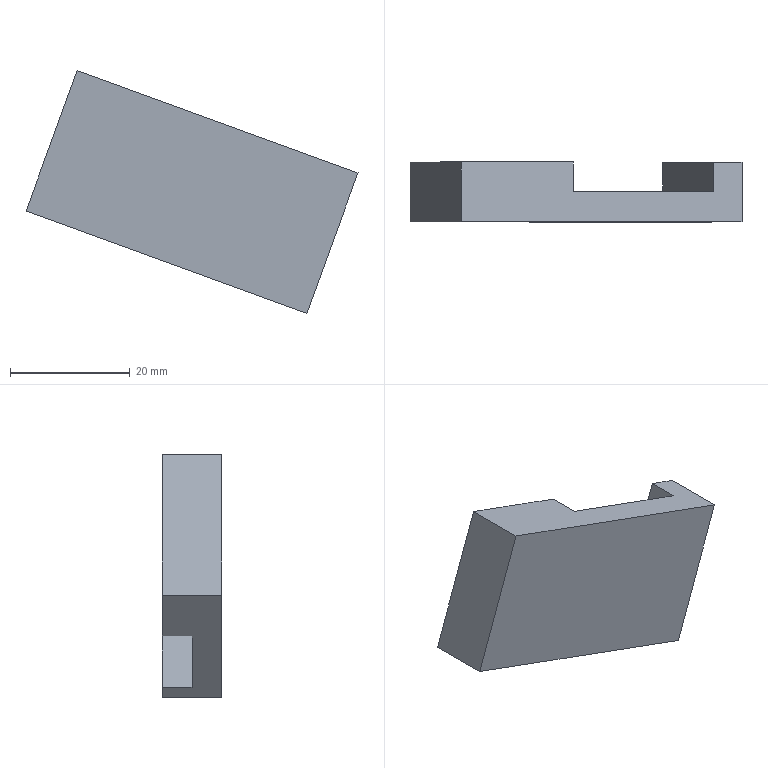Part | NX | features solid 2 | 1 solid | 10 faces | box 55.535 x 10 x 40.593 mm | volume 9375 mm3 | plane 10
STEP:
#1=CARTESIAN_POINT('',(816.611,435.,73.868));
#2=VERTEX_POINT('',#1);
#3=CARTESIAN_POINT('',(825.161,435.,97.361));
#4=VERTEX_POINT('',#3);
#5=CARTESIAN_POINT('',(822.425,435.,89.843));
#6=DIRECTION('',(-0.342,0.,-0.9397));
#7=VECTOR('',#6,1000.);
#8=LINE('',#5,#7);
#9=EDGE_CURVE('',#2,#4,#8,.F.);
#10=ORIENTED_EDGE('',*,*,#9,.T.);
#11=CARTESIAN_POINT('',(829.86,435.,95.651));
#12=VERTEX_POINT('',#11);
#13=CARTESIAN_POINT('',(782.875,435.,112.752));
#14=DIRECTION('',(-0.9397,0.,0.342));
#15=VECTOR('',#14,1000.);
#16=LINE('',#13,#15);
#17=EDGE_CURVE('',#4,#12,#16,.F.);
#18=ORIENTED_EDGE('',*,*,#17,.T.);
#19=CARTESIAN_POINT('',(821.309,435.,72.158));
#20=VERTEX_POINT('',#19);
#21=CARTESIAN_POINT('',(827.124,435.,88.133));
#22=DIRECTION('',(0.342,0.,0.9397));
#23=VECTOR('',#22,1000.);
#24=LINE('',#21,#23);
#25=EDGE_CURVE('',#12,#20,#24,.F.);
#26=ORIENTED_EDGE('',*,*,#25,.T.);
#27=CARTESIAN_POINT('',(774.325,435.,89.259));
#28=DIRECTION('',(-0.9397,0.,0.342));
#29=VECTOR('',#28,1000.);
#30=LINE('',#27,#29);
#31=EDGE_CURVE('',#2,#20,#30,.F.);
#32=ORIENTED_EDGE('',*,*,#31,.F.);
#33=EDGE_LOOP('',(#10,#18,#26,#32));
#34=FACE_BOUND('',#33,.T.);
#35=CARTESIAN_POINT('',(780.139,435.,105.234));
#36=DIRECTION('',(0.,-1.,0.));
#37=DIRECTION('',(0.9397,0.,-0.342));
#38=AXIS2_PLACEMENT_3D('',#35,#36,#37);
#39=PLANE('',#38);
#40=ADVANCED_FACE('',(#34),#39,.F.);
#41=CARTESIAN_POINT('',(782.875,425.,112.752));
#42=VERTEX_POINT('',#41);
#43=CARTESIAN_POINT('',(774.325,425.,89.259));
#44=VERTEX_POINT('',#43);
#45=CARTESIAN_POINT('',(780.139,425.,105.234));
#46=DIRECTION('',(-0.342,0.,-0.9397));
#47=VECTOR('',#46,1000.);
#48=LINE('',#45,#47);
#49=EDGE_CURVE('',#42,#44,#48,.T.);
#50=ORIENTED_EDGE('',*,*,#49,.T.);
#51=CARTESIAN_POINT('',(821.309,425.,72.158));
#52=VERTEX_POINT('',#51);
#53=CARTESIAN_POINT('',(774.325,425.,89.259));
#54=DIRECTION('',(0.9397,0.,-0.342));
#55=VECTOR('',#54,1000.);
#56=LINE('',#53,#55);
#57=EDGE_CURVE('',#44,#52,#56,.T.);
#58=ORIENTED_EDGE('',*,*,#57,.T.);
#59=CARTESIAN_POINT('',(829.86,425.,95.651));
#60=VERTEX_POINT('',#59);
#61=CARTESIAN_POINT('',(827.124,425.,88.133));
#62=DIRECTION('',(-0.342,0.,-0.9397));
#63=VECTOR('',#62,1000.);
#64=LINE('',#61,#63);
#65=EDGE_CURVE('',#60,#52,#64,.T.);
#66=ORIENTED_EDGE('',*,*,#65,.F.);
#67=CARTESIAN_POINT('',(782.875,425.,112.752));
#68=DIRECTION('',(0.9397,0.,-0.342));
#69=VECTOR('',#68,1000.);
#70=LINE('',#67,#69);
#71=EDGE_CURVE('',#42,#60,#70,.T.);
#72=ORIENTED_EDGE('',*,*,#71,.F.);
#73=EDGE_LOOP('',(#50,#58,#66,#72));
#74=FACE_BOUND('',#73,.T.);
#75=CARTESIAN_POINT('',(780.139,425.,105.234));
#76=DIRECTION('',(0.,-1.,0.));
#77=DIRECTION('',(0.9397,0.,-0.342));
#78=AXIS2_PLACEMENT_3D('',#75,#76,#77);
#79=PLANE('',#78);
#80=ADVANCED_FACE('',(#74),#79,.T.);
#81=ORIENTED_EDGE('',*,*,#65,.T.);
#82=CARTESIAN_POINT('',(821.309,425.,72.158));
#83=DIRECTION('',(0.,1.,0.));
#84=VECTOR('',#83,1000.);
#85=LINE('',#82,#84);
#86=EDGE_CURVE('',#52,#20,#85,.T.);
#87=ORIENTED_EDGE('',*,*,#86,.T.);
#88=ORIENTED_EDGE('',*,*,#25,.F.);
#89=CARTESIAN_POINT('',(829.86,425.,95.651));
#90=DIRECTION('',(0.,1.,0.));
#91=VECTOR('',#90,1000.);
#92=LINE('',#89,#91);
#93=EDGE_CURVE('',#60,#12,#92,.T.);
#94=ORIENTED_EDGE('',*,*,#93,.F.);
#95=EDGE_LOOP('',(#81,#87,#88,#94));
#96=FACE_BOUND('',#95,.T.);
#97=CARTESIAN_POINT('',(827.124,425.,88.133));
#98=DIRECTION('',(0.9397,0.,-0.342));
#99=DIRECTION('',(0.,1.,0.));
#100=AXIS2_PLACEMENT_3D('',#97,#98,#99);
#101=PLANE('',#100);
#102=ADVANCED_FACE('',(#96),#101,.T.);
#103=CARTESIAN_POINT('',(801.669,435.,105.911));
#104=VERTEX_POINT('',#103);
#105=CARTESIAN_POINT('',(793.119,435.,82.419));
#106=VERTEX_POINT('',#105);
#107=CARTESIAN_POINT('',(798.933,435.,98.394));
#108=DIRECTION('',(-0.342,0.,-0.9397));
#109=VECTOR('',#108,1000.);
#110=LINE('',#107,#109);
#111=EDGE_CURVE('',#104,#106,#110,.T.);
#112=ORIENTED_EDGE('',*,*,#111,.T.);
#113=CARTESIAN_POINT('',(774.325,435.,89.259));
#114=VERTEX_POINT('',#113);
#115=CARTESIAN_POINT('',(774.325,435.,89.259));
#116=DIRECTION('',(-0.9397,0.,0.342));
#117=VECTOR('',#116,1000.);
#118=LINE('',#115,#117);
#119=EDGE_CURVE('',#114,#106,#118,.F.);
#120=ORIENTED_EDGE('',*,*,#119,.F.);
#121=CARTESIAN_POINT('',(782.875,435.,112.752));
#122=VERTEX_POINT('',#121);
#123=CARTESIAN_POINT('',(780.139,435.,105.234));
#124=DIRECTION('',(-0.342,0.,-0.9397));
#125=VECTOR('',#124,1000.);
#126=LINE('',#123,#125);
#127=EDGE_CURVE('',#122,#114,#126,.T.);
#128=ORIENTED_EDGE('',*,*,#127,.F.);
#129=CARTESIAN_POINT('',(782.875,435.,112.752));
#130=DIRECTION('',(-0.9397,0.,0.342));
#131=VECTOR('',#130,1000.);
#132=LINE('',#129,#131);
#133=EDGE_CURVE('',#122,#104,#132,.F.);
#134=ORIENTED_EDGE('',*,*,#133,.T.);
#135=EDGE_LOOP('',(#112,#120,#128,#134));
#136=FACE_BOUND('',#135,.T.);
#137=CARTESIAN_POINT('',(780.139,435.,105.234));
#138=DIRECTION('',(0.,-1.,0.));
#139=DIRECTION('',(0.9397,0.,-0.342));
#140=AXIS2_PLACEMENT_3D('',#137,#138,#139);
#141=PLANE('',#140);
#142=ADVANCED_FACE('',(#136),#141,.F.);
#143=CARTESIAN_POINT('',(782.875,425.,112.752));
#144=DIRECTION('',(0.,1.,0.));
#145=VECTOR('',#144,1000.);
#146=LINE('',#143,#145);
#147=EDGE_CURVE('',#42,#122,#146,.T.);
#148=ORIENTED_EDGE('',*,*,#147,.T.);
#149=ORIENTED_EDGE('',*,*,#127,.T.);
#150=CARTESIAN_POINT('',(774.325,425.,89.259));
#151=DIRECTION('',(0.,-1.,0.));
#152=VECTOR('',#151,1000.);
#153=LINE('',#150,#152);
#154=EDGE_CURVE('',#44,#114,#153,.F.);
#155=ORIENTED_EDGE('',*,*,#154,.F.);
#156=ORIENTED_EDGE('',*,*,#49,.F.);
#157=EDGE_LOOP('',(#148,#149,#155,#156));
#158=FACE_BOUND('',#157,.T.);
#159=CARTESIAN_POINT('',(780.139,425.,105.234));
#160=DIRECTION('',(0.9397,0.,-0.342));
#161=DIRECTION('',(0.,1.,0.));
#162=AXIS2_PLACEMENT_3D('',#159,#160,#161);
#163=PLANE('',#162);
#164=ADVANCED_FACE('',(#158),#163,.F.);
#165=CARTESIAN_POINT('',(816.611,430.,73.868));
#166=VERTEX_POINT('',#165);
#167=CARTESIAN_POINT('',(816.611,425.,73.868));
#168=DIRECTION('',(0.,-1.,0.));
#169=VECTOR('',#168,1000.);
#170=LINE('',#167,#169);
#171=EDGE_CURVE('',#2,#166,#170,.T.);
#172=ORIENTED_EDGE('',*,*,#171,.F.);
#173=ORIENTED_EDGE('',*,*,#31,.T.);
#174=ORIENTED_EDGE('',*,*,#86,.F.);
#175=ORIENTED_EDGE('',*,*,#57,.F.);
#176=ORIENTED_EDGE('',*,*,#154,.T.);
#177=ORIENTED_EDGE('',*,*,#119,.T.);
#178=CARTESIAN_POINT('',(793.119,430.,82.419));
#179=VERTEX_POINT('',#178);
#180=CARTESIAN_POINT('',(793.119,425.,82.419));
#181=DIRECTION('',(0.,1.,0.));
#182=VECTOR('',#181,1000.);
#183=LINE('',#180,#182);
#184=EDGE_CURVE('',#106,#179,#183,.F.);
#185=ORIENTED_EDGE('',*,*,#184,.T.);
#186=CARTESIAN_POINT('',(774.325,430.,89.259));
#187=DIRECTION('',(-0.9397,0.,0.342));
#188=VECTOR('',#187,1000.);
#189=LINE('',#186,#188);
#190=EDGE_CURVE('',#166,#179,#189,.T.);
#191=ORIENTED_EDGE('',*,*,#190,.F.);
#192=EDGE_LOOP('',(#172,#173,#174,#175,#176,#177,#185,#191));
#193=FACE_BOUND('',#192,.T.);
#194=CARTESIAN_POINT('',(774.325,425.,89.259));
#195=DIRECTION('',(-0.342,0.,-0.9397));
#196=DIRECTION('',(0.9397,0.,-0.342));
#197=AXIS2_PLACEMENT_3D('',#194,#195,#196);
#198=PLANE('',#197);
#199=ADVANCED_FACE('',(#193),#198,.T.);
#200=CARTESIAN_POINT('',(825.161,430.,97.361));
#201=VERTEX_POINT('',#200);
#202=CARTESIAN_POINT('',(801.669,430.,105.911));
#203=VERTEX_POINT('',#202);
#204=CARTESIAN_POINT('',(810.596,430.,102.662));
#205=DIRECTION('',(-0.9397,0.,0.342));
#206=VECTOR('',#205,1000.);
#207=LINE('',#204,#206);
#208=EDGE_CURVE('',#201,#203,#207,.T.);
#209=ORIENTED_EDGE('',*,*,#208,.T.);
#210=CARTESIAN_POINT('',(801.669,425.,105.911));
#211=DIRECTION('',(0.,-1.,0.));
#212=VECTOR('',#211,1000.);
#213=LINE('',#210,#212);
#214=EDGE_CURVE('',#104,#203,#213,.T.);
#215=ORIENTED_EDGE('',*,*,#214,.F.);
#216=ORIENTED_EDGE('',*,*,#133,.F.);
#217=ORIENTED_EDGE('',*,*,#147,.F.);
#218=ORIENTED_EDGE('',*,*,#71,.T.);
#219=ORIENTED_EDGE('',*,*,#93,.T.);
#220=ORIENTED_EDGE('',*,*,#17,.F.);
#221=CARTESIAN_POINT('',(825.161,425.,97.361));
#222=DIRECTION('',(0.,-1.,0.));
#223=VECTOR('',#222,1000.);
#224=LINE('',#221,#223);
#225=EDGE_CURVE('',#4,#201,#224,.T.);
#226=ORIENTED_EDGE('',*,*,#225,.T.);
#227=EDGE_LOOP('',(#209,#215,#216,#217,#218,#219,#220,#226));
#228=FACE_BOUND('',#227,.T.);
#229=CARTESIAN_POINT('',(782.875,425.,112.752));
#230=DIRECTION('',(-0.342,0.,-0.9397));
#231=DIRECTION('',(0.9397,0.,-0.342));
#232=AXIS2_PLACEMENT_3D('',#229,#230,#231);
#233=PLANE('',#232);
#234=ADVANCED_FACE('',(#228),#233,.F.);
#235=ORIENTED_EDGE('',*,*,#9,.F.);
#236=ORIENTED_EDGE('',*,*,#171,.T.);
#237=CARTESIAN_POINT('',(825.161,430.,97.361));
#238=DIRECTION('',(-0.342,0.,-0.9397));
#239=VECTOR('',#238,1000.);
#240=LINE('',#237,#239);
#241=EDGE_CURVE('',#201,#166,#240,.T.);
#242=ORIENTED_EDGE('',*,*,#241,.F.);
#243=ORIENTED_EDGE('',*,*,#225,.F.);
#244=EDGE_LOOP('',(#235,#236,#242,#243));
#245=FACE_BOUND('',#244,.T.);
#246=CARTESIAN_POINT('',(825.161,425.,97.361));
#247=DIRECTION('',(0.9397,0.,-0.342));
#248=DIRECTION('',(-0.342,0.,-0.9397));
#249=AXIS2_PLACEMENT_3D('',#246,#247,#248);
#250=PLANE('',#249);
#251=ADVANCED_FACE('',(#245),#250,.F.);
#252=ORIENTED_EDGE('',*,*,#111,.F.);
#253=ORIENTED_EDGE('',*,*,#214,.T.);
#254=CARTESIAN_POINT('',(801.669,430.,105.911));
#255=DIRECTION('',(-0.342,0.,-0.9397));
#256=VECTOR('',#255,1000.);
#257=LINE('',#254,#256);
#258=EDGE_CURVE('',#203,#179,#257,.T.);
#259=ORIENTED_EDGE('',*,*,#258,.T.);
#260=ORIENTED_EDGE('',*,*,#184,.F.);
#261=EDGE_LOOP('',(#252,#253,#259,#260));
#262=FACE_BOUND('',#261,.T.);
#263=CARTESIAN_POINT('',(801.669,425.,105.911));
#264=DIRECTION('',(0.9397,0.,-0.342));
#265=DIRECTION('',(-0.342,0.,-0.9397));
#266=AXIS2_PLACEMENT_3D('',#263,#264,#265);
#267=PLANE('',#266);
#268=ADVANCED_FACE('',(#262),#267,.T.);
#269=ORIENTED_EDGE('',*,*,#258,.F.);
#270=ORIENTED_EDGE('',*,*,#208,.F.);
#271=ORIENTED_EDGE('',*,*,#241,.T.);
#272=ORIENTED_EDGE('',*,*,#190,.T.);
#273=EDGE_LOOP('',(#269,#270,#271,#272));
#274=FACE_BOUND('',#273,.T.);
#275=CARTESIAN_POINT('',(810.596,430.,102.662));
#276=DIRECTION('',(0.,-1.,0.));
#277=DIRECTION('',(0.766,0.,-0.6428));
#278=AXIS2_PLACEMENT_3D('',#275,#276,#277);
#279=PLANE('',#278);
#280=ADVANCED_FACE('',(#274),#279,.F.);
#281=CLOSED_SHELL('',(#40,#80,#102,#142,#164,#199,#234,#251,#268,#280));
#282=MANIFOLD_SOLID_BREP('',#281);
#283=(LENGTH_UNIT()NAMED_UNIT(*)SI_UNIT(.MILLI.,.METRE.));
#284=UNCERTAINTY_MEASURE_WITH_UNIT(LENGTH_MEASURE(0.00001),#283,'','');
#285=(NAMED_UNIT(*)PLANE_ANGLE_UNIT()SI_UNIT($,.RADIAN.));
#286=(NAMED_UNIT(*)SI_UNIT($,.STERADIAN.)SOLID_ANGLE_UNIT());
#287=(GEOMETRIC_REPRESENTATION_CONTEXT(3)GLOBAL_UNCERTAINTY_ASSIGNED_CONTEXT((#284))GLOBAL_UNIT_ASSIGNED_CONTEXT((#283,#285,#286))REPRESENTATION_CONTEXT('',''));
#288=ADVANCED_BREP_SHAPE_REPRESENTATION('',(#282),#287);